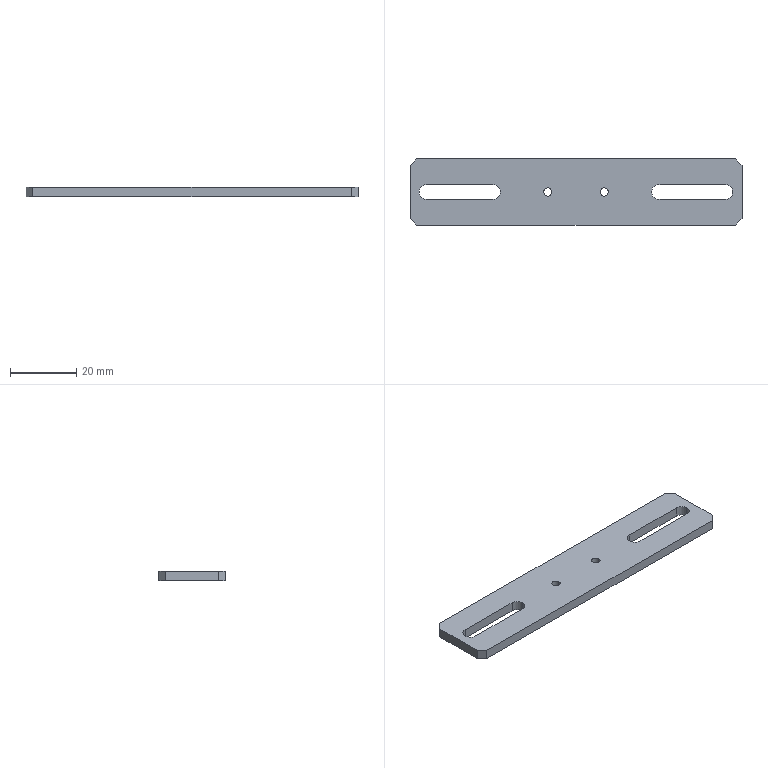Part | SolidWorks | features Chamfer 1, Cut 1, FlatPattern 1, HoleWzd 1, SMBaseFlange 1, SheetMetal 1 | 1 solid | 24 faces | box 100 x 20 x 3 mm | volume 5311 mm3 | plane 14 | cylinder 10 | commonest cylinder face diameters 4.5 x6 2.5 x4
STEP:
#1=CARTESIAN_POINT('',(-22.75,0.,-3.));
#2=VERTEX_POINT('',#1);
#3=CARTESIAN_POINT('',(-25.,2.25,-3.));
#4=VERTEX_POINT('',#3);
#5=CARTESIAN_POINT('',(-25.,0.,-3.));
#6=DIRECTION('',(0.,0.,1.));
#7=DIRECTION('',(1.,0.,0.));
#8=AXIS2_PLACEMENT_3D('',#5,#6,#7);
#9=CIRCLE('',#8,2.25);
#10=EDGE_CURVE('',#2,#4,#9,.T.);
#11=ORIENTED_EDGE('',*,*,#10,.F.);
#12=CARTESIAN_POINT('',(-22.75,0.,0.));
#13=VERTEX_POINT('',#12);
#14=CARTESIAN_POINT('',(-22.75,0.,-3.));
#15=DIRECTION('',(0.,0.,1.));
#16=VECTOR('',#15,1000.);
#17=LINE('',#14,#16);
#18=EDGE_CURVE('',#2,#13,#17,.T.);
#19=ORIENTED_EDGE('',*,*,#18,.T.);
#20=CARTESIAN_POINT('',(-25.,2.25,0.));
#21=VERTEX_POINT('',#20);
#22=CARTESIAN_POINT('',(-25.,0.,0.));
#23=DIRECTION('',(0.,0.,1.));
#24=DIRECTION('',(1.,0.,0.));
#25=AXIS2_PLACEMENT_3D('',#22,#23,#24);
#26=CIRCLE('',#25,2.25);
#27=EDGE_CURVE('',#13,#21,#26,.T.);
#28=ORIENTED_EDGE('',*,*,#27,.T.);
#29=CARTESIAN_POINT('',(-25.,2.25,-3.));
#30=DIRECTION('',(0.,0.,1.));
#31=VECTOR('',#30,1000.);
#32=LINE('',#29,#31);
#33=EDGE_CURVE('',#4,#21,#32,.T.);
#34=ORIENTED_EDGE('',*,*,#33,.F.);
#35=EDGE_LOOP('',(#11,#19,#28,#34));
#36=FACE_OUTER_BOUND('',#35,.T.);
#37=CARTESIAN_POINT('',(-25.,0.,-3.));
#38=DIRECTION('',(0.,0.,1.));
#39=DIRECTION('',(1.,0.,0.));
#40=AXIS2_PLACEMENT_3D('',#37,#38,#39);
#41=CYLINDRICAL_SURFACE('',#40,2.25);
#42=ADVANCED_FACE('',(#36),#41,.F.);
#43=CARTESIAN_POINT('',(47.25,0.,-3.));
#44=VERTEX_POINT('',#43);
#45=CARTESIAN_POINT('',(45.,2.25,-3.));
#46=VERTEX_POINT('',#45);
#47=CARTESIAN_POINT('',(45.,0.,-3.));
#48=DIRECTION('',(0.,0.,1.));
#49=DIRECTION('',(1.,0.,0.));
#50=AXIS2_PLACEMENT_3D('',#47,#48,#49);
#51=CIRCLE('',#50,2.25);
#52=EDGE_CURVE('',#44,#46,#51,.T.);
#53=ORIENTED_EDGE('',*,*,#52,.F.);
#54=CARTESIAN_POINT('',(47.25,0.,0.));
#55=VERTEX_POINT('',#54);
#56=CARTESIAN_POINT('',(47.25,0.,-3.));
#57=DIRECTION('',(0.,0.,1.));
#58=VECTOR('',#57,1000.);
#59=LINE('',#56,#58);
#60=EDGE_CURVE('',#44,#55,#59,.T.);
#61=ORIENTED_EDGE('',*,*,#60,.T.);
#62=CARTESIAN_POINT('',(45.,2.25,0.));
#63=VERTEX_POINT('',#62);
#64=CARTESIAN_POINT('',(45.,0.,0.));
#65=DIRECTION('',(0.,0.,1.));
#66=DIRECTION('',(1.,0.,0.));
#67=AXIS2_PLACEMENT_3D('',#64,#65,#66);
#68=CIRCLE('',#67,2.25);
#69=EDGE_CURVE('',#55,#63,#68,.T.);
#70=ORIENTED_EDGE('',*,*,#69,.T.);
#71=CARTESIAN_POINT('',(45.,2.25,-3.));
#72=DIRECTION('',(0.,0.,1.));
#73=VECTOR('',#72,1000.);
#74=LINE('',#71,#73);
#75=EDGE_CURVE('',#46,#63,#74,.T.);
#76=ORIENTED_EDGE('',*,*,#75,.F.);
#77=EDGE_LOOP('',(#53,#61,#70,#76));
#78=FACE_OUTER_BOUND('',#77,.T.);
#79=CARTESIAN_POINT('',(45.,0.,-3.));
#80=DIRECTION('',(0.,0.,1.));
#81=DIRECTION('',(1.,0.,0.));
#82=AXIS2_PLACEMENT_3D('',#79,#80,#81);
#83=CYLINDRICAL_SURFACE('',#82,2.25);
#84=ADVANCED_FACE('',(#78),#83,.F.);
#85=CARTESIAN_POINT('',(7.25,0.,-3.));
#86=VERTEX_POINT('',#85);
#87=CARTESIAN_POINT('',(9.75,0.,-3.));
#88=VERTEX_POINT('',#87);
#89=CARTESIAN_POINT('',(8.5,0.,-3.));
#90=DIRECTION('',(0.,0.,1.));
#91=DIRECTION('',(1.,0.,0.));
#92=AXIS2_PLACEMENT_3D('',#89,#90,#91);
#93=CIRCLE('',#92,1.25);
#94=EDGE_CURVE('',#86,#88,#93,.T.);
#95=ORIENTED_EDGE('',*,*,#94,.F.);
#96=CARTESIAN_POINT('',(7.25,0.,0.));
#97=VERTEX_POINT('',#96);
#98=CARTESIAN_POINT('',(7.25,0.,0.));
#99=DIRECTION('',(0.,0.,1.));
#100=VECTOR('',#99,1000.);
#101=LINE('',#98,#100);
#102=EDGE_CURVE('',#86,#97,#101,.T.);
#103=ORIENTED_EDGE('',*,*,#102,.T.);
#104=CARTESIAN_POINT('',(9.75,0.,0.));
#105=VERTEX_POINT('',#104);
#106=CARTESIAN_POINT('',(8.5,0.,0.));
#107=DIRECTION('',(0.,0.,1.));
#108=DIRECTION('',(1.,0.,0.));
#109=AXIS2_PLACEMENT_3D('',#106,#107,#108);
#110=CIRCLE('',#109,1.25);
#111=EDGE_CURVE('',#97,#105,#110,.T.);
#112=ORIENTED_EDGE('',*,*,#111,.T.);
#113=CARTESIAN_POINT('',(9.75,0.,0.));
#114=DIRECTION('',(0.,0.,1.));
#115=VECTOR('',#114,1000.);
#116=LINE('',#113,#115);
#117=EDGE_CURVE('',#88,#105,#116,.T.);
#118=ORIENTED_EDGE('',*,*,#117,.F.);
#119=EDGE_LOOP('',(#95,#103,#112,#118));
#120=FACE_OUTER_BOUND('',#119,.T.);
#121=CARTESIAN_POINT('',(8.5,0.,0.));
#122=DIRECTION('',(0.,0.,1.));
#123=DIRECTION('',(1.,0.,0.));
#124=AXIS2_PLACEMENT_3D('',#121,#122,#123);
#125=CYLINDRICAL_SURFACE('',#124,1.25);
#126=ADVANCED_FACE('',(#120),#125,.F.);
#127=CARTESIAN_POINT('',(-9.75,0.,-3.));
#128=VERTEX_POINT('',#127);
#129=CARTESIAN_POINT('',(-7.25,0.,-3.));
#130=VERTEX_POINT('',#129);
#131=CARTESIAN_POINT('',(-8.5,0.,-3.));
#132=DIRECTION('',(0.,0.,1.));
#133=DIRECTION('',(1.,0.,0.));
#134=AXIS2_PLACEMENT_3D('',#131,#132,#133);
#135=CIRCLE('',#134,1.25);
#136=EDGE_CURVE('',#128,#130,#135,.T.);
#137=ORIENTED_EDGE('',*,*,#136,.F.);
#138=CARTESIAN_POINT('',(-9.75,0.,0.));
#139=VERTEX_POINT('',#138);
#140=CARTESIAN_POINT('',(-9.75,0.,0.));
#141=DIRECTION('',(0.,0.,1.));
#142=VECTOR('',#141,1000.);
#143=LINE('',#140,#142);
#144=EDGE_CURVE('',#128,#139,#143,.T.);
#145=ORIENTED_EDGE('',*,*,#144,.T.);
#146=CARTESIAN_POINT('',(-7.25,0.,0.));
#147=VERTEX_POINT('',#146);
#148=CARTESIAN_POINT('',(-8.5,0.,0.));
#149=DIRECTION('',(0.,0.,1.));
#150=DIRECTION('',(1.,0.,0.));
#151=AXIS2_PLACEMENT_3D('',#148,#149,#150);
#152=CIRCLE('',#151,1.25);
#153=EDGE_CURVE('',#139,#147,#152,.T.);
#154=ORIENTED_EDGE('',*,*,#153,.T.);
#155=CARTESIAN_POINT('',(-7.25,0.,0.));
#156=DIRECTION('',(0.,0.,1.));
#157=VECTOR('',#156,1000.);
#158=LINE('',#155,#157);
#159=EDGE_CURVE('',#130,#147,#158,.T.);
#160=ORIENTED_EDGE('',*,*,#159,.F.);
#161=EDGE_LOOP('',(#137,#145,#154,#160));
#162=FACE_OUTER_BOUND('',#161,.T.);
#163=CARTESIAN_POINT('',(-8.5,0.,0.));
#164=DIRECTION('',(0.,0.,1.));
#165=DIRECTION('',(1.,0.,0.));
#166=AXIS2_PLACEMENT_3D('',#163,#164,#165);
#167=CYLINDRICAL_SURFACE('',#166,1.25);
#168=ADVANCED_FACE('',(#162),#167,.F.);
#169=CARTESIAN_POINT('',(50.,-8.,-3.));
#170=VERTEX_POINT('',#169);
#171=CARTESIAN_POINT('',(50.,8.,-3.));
#172=VERTEX_POINT('',#171);
#173=CARTESIAN_POINT('',(50.,10.,-3.));
#174=DIRECTION('',(0.,1.,0.));
#175=VECTOR('',#174,1000.);
#176=LINE('',#173,#175);
#177=EDGE_CURVE('',#170,#172,#176,.T.);
#178=ORIENTED_EDGE('',*,*,#177,.T.);
#179=CARTESIAN_POINT('',(50.,8.,0.));
#180=VERTEX_POINT('',#179);
#181=CARTESIAN_POINT('',(50.,8.,-3.));
#182=DIRECTION('',(0.,0.,1.));
#183=VECTOR('',#182,1000.);
#184=LINE('',#181,#183);
#185=EDGE_CURVE('',#172,#180,#184,.T.);
#186=ORIENTED_EDGE('',*,*,#185,.T.);
#187=CARTESIAN_POINT('',(50.,-8.,0.));
#188=VERTEX_POINT('',#187);
#189=CARTESIAN_POINT('',(50.,10.,0.));
#190=DIRECTION('',(0.,1.,0.));
#191=VECTOR('',#190,1000.);
#192=LINE('',#189,#191);
#193=EDGE_CURVE('',#188,#180,#192,.T.);
#194=ORIENTED_EDGE('',*,*,#193,.F.);
#195=CARTESIAN_POINT('',(50.,-8.,-3.));
#196=DIRECTION('',(0.,0.,-1.));
#197=VECTOR('',#196,1000.);
#198=LINE('',#195,#197);
#199=EDGE_CURVE('',#188,#170,#198,.T.);
#200=ORIENTED_EDGE('',*,*,#199,.T.);
#201=EDGE_LOOP('',(#178,#186,#194,#200));
#202=FACE_OUTER_BOUND('',#201,.T.);
#203=CARTESIAN_POINT('',(50.,10.,-3.));
#204=DIRECTION('',(1.,0.,0.));
#205=DIRECTION('',(0.,0.,-1.));
#206=AXIS2_PLACEMENT_3D('',#203,#204,#205);
#207=PLANE('',#206);
#208=ADVANCED_FACE('',(#202),#207,.T.);
#209=CARTESIAN_POINT('',(-48.,-10.,-3.));
#210=VERTEX_POINT('',#209);
#211=CARTESIAN_POINT('',(48.,-10.,-3.));
#212=VERTEX_POINT('',#211);
#213=CARTESIAN_POINT('',(-50.,-10.,-3.));
#214=DIRECTION('',(1.,0.,0.));
#215=VECTOR('',#214,1000.);
#216=LINE('',#213,#215);
#217=EDGE_CURVE('',#210,#212,#216,.T.);
#218=ORIENTED_EDGE('',*,*,#217,.T.);
#219=CARTESIAN_POINT('',(48.,-10.,0.));
#220=VERTEX_POINT('',#219);
#221=CARTESIAN_POINT('',(48.,-10.,-3.));
#222=DIRECTION('',(0.,0.,1.));
#223=VECTOR('',#222,1000.);
#224=LINE('',#221,#223);
#225=EDGE_CURVE('',#212,#220,#224,.T.);
#226=ORIENTED_EDGE('',*,*,#225,.T.);
#227=CARTESIAN_POINT('',(-48.,-10.,0.));
#228=VERTEX_POINT('',#227);
#229=CARTESIAN_POINT('',(-50.,-10.,0.));
#230=DIRECTION('',(1.,0.,0.));
#231=VECTOR('',#230,1000.);
#232=LINE('',#229,#231);
#233=EDGE_CURVE('',#228,#220,#232,.T.);
#234=ORIENTED_EDGE('',*,*,#233,.F.);
#235=CARTESIAN_POINT('',(-48.,-10.,-3.));
#236=DIRECTION('',(0.,0.,-1.));
#237=VECTOR('',#236,1000.);
#238=LINE('',#235,#237);
#239=EDGE_CURVE('',#228,#210,#238,.T.);
#240=ORIENTED_EDGE('',*,*,#239,.T.);
#241=EDGE_LOOP('',(#218,#226,#234,#240));
#242=FACE_OUTER_BOUND('',#241,.T.);
#243=CARTESIAN_POINT('',(-50.,-10.,-3.));
#244=DIRECTION('',(0.,-1.,0.));
#245=DIRECTION('',(0.,0.,-1.));
#246=AXIS2_PLACEMENT_3D('',#243,#244,#245);
#247=PLANE('',#246);
#248=ADVANCED_FACE('',(#242),#247,.T.);
#249=CARTESIAN_POINT('',(-50.,8.,0.));
#250=VERTEX_POINT('',#249);
#251=CARTESIAN_POINT('',(-50.,-8.,0.));
#252=VERTEX_POINT('',#251);
#253=CARTESIAN_POINT('',(-50.,10.,0.));
#254=DIRECTION('',(0.,-1.,0.));
#255=VECTOR('',#254,1000.);
#256=LINE('',#253,#255);
#257=EDGE_CURVE('',#250,#252,#256,.T.);
#258=ORIENTED_EDGE('',*,*,#257,.F.);
#259=CARTESIAN_POINT('',(-50.,8.,-3.));
#260=VERTEX_POINT('',#259);
#261=CARTESIAN_POINT('',(-50.,8.,-3.));
#262=DIRECTION('',(0.,0.,-1.));
#263=VECTOR('',#262,1000.);
#264=LINE('',#261,#263);
#265=EDGE_CURVE('',#250,#260,#264,.T.);
#266=ORIENTED_EDGE('',*,*,#265,.T.);
#267=CARTESIAN_POINT('',(-50.,-8.,-3.));
#268=VERTEX_POINT('',#267);
#269=CARTESIAN_POINT('',(-50.,10.,-3.));
#270=DIRECTION('',(0.,-1.,0.));
#271=VECTOR('',#270,1000.);
#272=LINE('',#269,#271);
#273=EDGE_CURVE('',#260,#268,#272,.T.);
#274=ORIENTED_EDGE('',*,*,#273,.T.);
#275=CARTESIAN_POINT('',(-50.,-8.,-3.));
#276=DIRECTION('',(0.,0.,1.));
#277=VECTOR('',#276,1000.);
#278=LINE('',#275,#277);
#279=EDGE_CURVE('',#268,#252,#278,.T.);
#280=ORIENTED_EDGE('',*,*,#279,.T.);
#281=EDGE_LOOP('',(#258,#266,#274,#280));
#282=FACE_OUTER_BOUND('',#281,.T.);
#283=CARTESIAN_POINT('',(-50.,10.,-3.));
#284=DIRECTION('',(-1.,0.,0.));
#285=DIRECTION('',(0.,0.,1.));
#286=AXIS2_PLACEMENT_3D('',#283,#284,#285);
#287=PLANE('',#286);
#288=ADVANCED_FACE('',(#282),#287,.T.);
#289=CARTESIAN_POINT('',(48.,10.,0.));
#290=VERTEX_POINT('',#289);
#291=CARTESIAN_POINT('',(-48.,10.,0.));
#292=VERTEX_POINT('',#291);
#293=CARTESIAN_POINT('',(-50.,10.,0.));
#294=DIRECTION('',(-1.,0.,0.));
#295=VECTOR('',#294,1000.);
#296=LINE('',#293,#295);
#297=EDGE_CURVE('',#290,#292,#296,.T.);
#298=ORIENTED_EDGE('',*,*,#297,.F.);
#299=CARTESIAN_POINT('',(48.,10.,-3.));
#300=VERTEX_POINT('',#299);
#301=CARTESIAN_POINT('',(48.,10.,-3.));
#302=DIRECTION('',(0.,0.,-1.));
#303=VECTOR('',#302,1000.);
#304=LINE('',#301,#303);
#305=EDGE_CURVE('',#290,#300,#304,.T.);
#306=ORIENTED_EDGE('',*,*,#305,.T.);
#307=CARTESIAN_POINT('',(-48.,10.,-3.));
#308=VERTEX_POINT('',#307);
#309=CARTESIAN_POINT('',(-50.,10.,-3.));
#310=DIRECTION('',(-1.,0.,0.));
#311=VECTOR('',#310,1000.);
#312=LINE('',#309,#311);
#313=EDGE_CURVE('',#300,#308,#312,.T.);
#314=ORIENTED_EDGE('',*,*,#313,.T.);
#315=CARTESIAN_POINT('',(-48.,10.,-3.));
#316=DIRECTION('',(0.,0.,1.));
#317=VECTOR('',#316,1000.);
#318=LINE('',#315,#317);
#319=EDGE_CURVE('',#308,#292,#318,.T.);
#320=ORIENTED_EDGE('',*,*,#319,.T.);
#321=EDGE_LOOP('',(#298,#306,#314,#320));
#322=FACE_OUTER_BOUND('',#321,.T.);
#323=CARTESIAN_POINT('',(-50.,10.,-3.));
#324=DIRECTION('',(0.,1.,0.));
#325=DIRECTION('',(0.,0.,1.));
#326=AXIS2_PLACEMENT_3D('',#323,#324,#325);
#327=PLANE('',#326);
#328=ADVANCED_FACE('',(#322),#327,.T.);
#329=CARTESIAN_POINT('',(-45.,-2.25,-3.));
#330=VERTEX_POINT('',#329);
#331=CARTESIAN_POINT('',(-25.,-2.25,-3.));
#332=VERTEX_POINT('',#331);
#333=CARTESIAN_POINT('',(-25.,-2.25,-3.));
#334=DIRECTION('',(1.,0.,0.));
#335=VECTOR('',#334,1000.);
#336=LINE('',#333,#335);
#337=EDGE_CURVE('',#330,#332,#336,.T.);
#338=ORIENTED_EDGE('',*,*,#337,.T.);
#339=CARTESIAN_POINT('',(-25.,0.,-3.));
#340=DIRECTION('',(0.,0.,1.));
#341=DIRECTION('',(1.,0.,0.));
#342=AXIS2_PLACEMENT_3D('',#339,#340,#341);
#343=CIRCLE('',#342,2.25);
#344=EDGE_CURVE('',#332,#2,#343,.T.);
#345=ORIENTED_EDGE('',*,*,#344,.T.);
#346=ORIENTED_EDGE('',*,*,#10,.T.);
#347=CARTESIAN_POINT('',(-45.,2.25,-3.));
#348=VERTEX_POINT('',#347);
#349=CARTESIAN_POINT('',(-25.,2.25,-3.));
#350=DIRECTION('',(-1.,0.,0.));
#351=VECTOR('',#350,1000.);
#352=LINE('',#349,#351);
#353=EDGE_CURVE('',#4,#348,#352,.T.);
#354=ORIENTED_EDGE('',*,*,#353,.T.);
#355=CARTESIAN_POINT('',(-45.,0.,-3.));
#356=DIRECTION('',(0.,0.,1.));
#357=DIRECTION('',(1.,0.,0.));
#358=AXIS2_PLACEMENT_3D('',#355,#356,#357);
#359=CIRCLE('',#358,2.25);
#360=EDGE_CURVE('',#348,#330,#359,.T.);
#361=ORIENTED_EDGE('',*,*,#360,.T.);
#362=EDGE_LOOP('',(#338,#345,#346,#354,#361));
#363=FACE_BOUND('',#362,.T.);
#364=CARTESIAN_POINT('',(25.,-2.25,-3.));
#365=VERTEX_POINT('',#364);
#366=CARTESIAN_POINT('',(45.,-2.25,-3.));
#367=VERTEX_POINT('',#366);
#368=CARTESIAN_POINT('',(45.,-2.25,-3.));
#369=DIRECTION('',(1.,0.,0.));
#370=VECTOR('',#369,1000.);
#371=LINE('',#368,#370);
#372=EDGE_CURVE('',#365,#367,#371,.T.);
#373=ORIENTED_EDGE('',*,*,#372,.T.);
#374=CARTESIAN_POINT('',(45.,0.,-3.));
#375=DIRECTION('',(0.,0.,1.));
#376=DIRECTION('',(1.,0.,0.));
#377=AXIS2_PLACEMENT_3D('',#374,#375,#376);
#378=CIRCLE('',#377,2.25);
#379=EDGE_CURVE('',#367,#44,#378,.T.);
#380=ORIENTED_EDGE('',*,*,#379,.T.);
#381=ORIENTED_EDGE('',*,*,#52,.T.);
#382=CARTESIAN_POINT('',(25.,2.25,-3.));
#383=VERTEX_POINT('',#382);
#384=CARTESIAN_POINT('',(45.,2.25,-3.));
#385=DIRECTION('',(-1.,0.,0.));
#386=VECTOR('',#385,1000.);
#387=LINE('',#384,#386);
#388=EDGE_CURVE('',#46,#383,#387,.T.);
#389=ORIENTED_EDGE('',*,*,#388,.T.);
#390=CARTESIAN_POINT('',(25.,0.,-3.));
#391=DIRECTION('',(0.,0.,1.));
#392=DIRECTION('',(1.,0.,0.));
#393=AXIS2_PLACEMENT_3D('',#390,#391,#392);
#394=CIRCLE('',#393,2.25);
#395=EDGE_CURVE('',#383,#365,#394,.T.);
#396=ORIENTED_EDGE('',*,*,#395,.T.);
#397=EDGE_LOOP('',(#373,#380,#381,#389,#396));
#398=FACE_BOUND('',#397,.T.);
#399=CARTESIAN_POINT('',(8.5,0.,-3.));
#400=DIRECTION('',(0.,0.,1.));
#401=DIRECTION('',(1.,0.,0.));
#402=AXIS2_PLACEMENT_3D('',#399,#400,#401);
#403=CIRCLE('',#402,1.25);
#404=EDGE_CURVE('',#88,#86,#403,.T.);
#405=ORIENTED_EDGE('',*,*,#404,.T.);
#406=ORIENTED_EDGE('',*,*,#94,.T.);
#407=EDGE_LOOP('',(#405,#406));
#408=FACE_BOUND('',#407,.T.);
#409=CARTESIAN_POINT('',(-8.5,0.,-3.));
#410=DIRECTION('',(0.,0.,1.));
#411=DIRECTION('',(1.,0.,0.));
#412=AXIS2_PLACEMENT_3D('',#409,#410,#411);
#413=CIRCLE('',#412,1.25);
#414=EDGE_CURVE('',#130,#128,#413,.T.);
#415=ORIENTED_EDGE('',*,*,#414,.T.);
#416=ORIENTED_EDGE('',*,*,#136,.T.);
#417=EDGE_LOOP('',(#415,#416));
#418=FACE_BOUND('',#417,.T.);
#419=ORIENTED_EDGE('',*,*,#313,.F.);
#420=CARTESIAN_POINT('',(50.,8.,-3.));
#421=DIRECTION('',(0.7071,-0.7071,0.));
#422=VECTOR('',#421,1000.);
#423=LINE('',#420,#422);
#424=EDGE_CURVE('',#300,#172,#423,.T.);
#425=ORIENTED_EDGE('',*,*,#424,.T.);
#426=ORIENTED_EDGE('',*,*,#177,.F.);
#427=CARTESIAN_POINT('',(48.,-10.,-3.));
#428=DIRECTION('',(-0.7071,-0.7071,0.));
#429=VECTOR('',#428,1000.);
#430=LINE('',#427,#429);
#431=EDGE_CURVE('',#170,#212,#430,.T.);
#432=ORIENTED_EDGE('',*,*,#431,.T.);
#433=ORIENTED_EDGE('',*,*,#217,.F.);
#434=CARTESIAN_POINT('',(-50.,-8.,-3.));
#435=DIRECTION('',(-0.7071,0.7071,0.));
#436=VECTOR('',#435,1000.);
#437=LINE('',#434,#436);
#438=EDGE_CURVE('',#210,#268,#437,.T.);
#439=ORIENTED_EDGE('',*,*,#438,.T.);
#440=ORIENTED_EDGE('',*,*,#273,.F.);
#441=CARTESIAN_POINT('',(-48.,10.,-3.));
#442=DIRECTION('',(0.7071,0.7071,0.));
#443=VECTOR('',#442,1000.);
#444=LINE('',#441,#443);
#445=EDGE_CURVE('',#260,#308,#444,.T.);
#446=ORIENTED_EDGE('',*,*,#445,.T.);
#447=EDGE_LOOP('',(#419,#425,#426,#432,#433,#439,#440,#446));
#448=FACE_OUTER_BOUND('',#447,.T.);
#449=CARTESIAN_POINT('',(0.,0.,-3.));
#450=DIRECTION('',(0.,0.,1.));
#451=DIRECTION('',(1.,0.,0.));
#452=AXIS2_PLACEMENT_3D('',#449,#450,#451);
#453=PLANE('',#452);
#454=ADVANCED_FACE('',(#363,#398,#408,#418,#448),#453,.F.);
#455=CARTESIAN_POINT('',(-25.,-2.25,0.));
#456=VERTEX_POINT('',#455);
#457=CARTESIAN_POINT('',(-25.,0.,0.));
#458=DIRECTION('',(0.,0.,1.));
#459=DIRECTION('',(1.,0.,0.));
#460=AXIS2_PLACEMENT_3D('',#457,#458,#459);
#461=CIRCLE('',#460,2.25);
#462=EDGE_CURVE('',#456,#13,#461,.T.);
#463=ORIENTED_EDGE('',*,*,#462,.F.);
#464=CARTESIAN_POINT('',(-45.,-2.25,0.));
#465=VERTEX_POINT('',#464);
#466=CARTESIAN_POINT('',(-25.,-2.25,0.));
#467=DIRECTION('',(1.,0.,0.));
#468=VECTOR('',#467,1000.);
#469=LINE('',#466,#468);
#470=EDGE_CURVE('',#465,#456,#469,.T.);
#471=ORIENTED_EDGE('',*,*,#470,.F.);
#472=CARTESIAN_POINT('',(-45.,2.25,0.));
#473=VERTEX_POINT('',#472);
#474=CARTESIAN_POINT('',(-45.,0.,0.));
#475=DIRECTION('',(0.,0.,1.));
#476=DIRECTION('',(1.,0.,0.));
#477=AXIS2_PLACEMENT_3D('',#474,#475,#476);
#478=CIRCLE('',#477,2.25);
#479=EDGE_CURVE('',#473,#465,#478,.T.);
#480=ORIENTED_EDGE('',*,*,#479,.F.);
#481=CARTESIAN_POINT('',(-25.,2.25,0.));
#482=DIRECTION('',(-1.,0.,0.));
#483=VECTOR('',#482,1000.);
#484=LINE('',#481,#483);
#485=EDGE_CURVE('',#21,#473,#484,.T.);
#486=ORIENTED_EDGE('',*,*,#485,.F.);
#487=ORIENTED_EDGE('',*,*,#27,.F.);
#488=EDGE_LOOP('',(#463,#471,#480,#486,#487));
#489=FACE_BOUND('',#488,.T.);
#490=CARTESIAN_POINT('',(45.,-2.25,0.));
#491=VERTEX_POINT('',#490);
#492=CARTESIAN_POINT('',(45.,0.,0.));
#493=DIRECTION('',(0.,0.,1.));
#494=DIRECTION('',(1.,0.,0.));
#495=AXIS2_PLACEMENT_3D('',#492,#493,#494);
#496=CIRCLE('',#495,2.25);
#497=EDGE_CURVE('',#491,#55,#496,.T.);
#498=ORIENTED_EDGE('',*,*,#497,.F.);
#499=CARTESIAN_POINT('',(25.,-2.25,0.));
#500=VERTEX_POINT('',#499);
#501=CARTESIAN_POINT('',(45.,-2.25,0.));
#502=DIRECTION('',(1.,0.,0.));
#503=VECTOR('',#502,1000.);
#504=LINE('',#501,#503);
#505=EDGE_CURVE('',#500,#491,#504,.T.);
#506=ORIENTED_EDGE('',*,*,#505,.F.);
#507=CARTESIAN_POINT('',(25.,2.25,0.));
#508=VERTEX_POINT('',#507);
#509=CARTESIAN_POINT('',(25.,0.,0.));
#510=DIRECTION('',(0.,0.,1.));
#511=DIRECTION('',(1.,0.,0.));
#512=AXIS2_PLACEMENT_3D('',#509,#510,#511);
#513=CIRCLE('',#512,2.25);
#514=EDGE_CURVE('',#508,#500,#513,.T.);
#515=ORIENTED_EDGE('',*,*,#514,.F.);
#516=CARTESIAN_POINT('',(45.,2.25,0.));
#517=DIRECTION('',(-1.,0.,0.));
#518=VECTOR('',#517,1000.);
#519=LINE('',#516,#518);
#520=EDGE_CURVE('',#63,#508,#519,.T.);
#521=ORIENTED_EDGE('',*,*,#520,.F.);
#522=ORIENTED_EDGE('',*,*,#69,.F.);
#523=EDGE_LOOP('',(#498,#506,#515,#521,#522));
#524=FACE_BOUND('',#523,.T.);
#525=CARTESIAN_POINT('',(8.5,0.,0.));
#526=DIRECTION('',(0.,0.,1.));
#527=DIRECTION('',(1.,0.,0.));
#528=AXIS2_PLACEMENT_3D('',#525,#526,#527);
#529=CIRCLE('',#528,1.25);
#530=EDGE_CURVE('',#105,#97,#529,.T.);
#531=ORIENTED_EDGE('',*,*,#530,.F.);
#532=ORIENTED_EDGE('',*,*,#111,.F.);
#533=EDGE_LOOP('',(#531,#532));
#534=FACE_BOUND('',#533,.T.);
#535=CARTESIAN_POINT('',(-8.5,0.,0.));
#536=DIRECTION('',(0.,0.,1.));
#537=DIRECTION('',(1.,0.,0.));
#538=AXIS2_PLACEMENT_3D('',#535,#536,#537);
#539=CIRCLE('',#538,1.25);
#540=EDGE_CURVE('',#147,#139,#539,.T.);
#541=ORIENTED_EDGE('',*,*,#540,.F.);
#542=ORIENTED_EDGE('',*,*,#153,.F.);
#543=EDGE_LOOP('',(#541,#542));
#544=FACE_BOUND('',#543,.T.);
#545=ORIENTED_EDGE('',*,*,#193,.T.);
#546=CARTESIAN_POINT('',(29.,29.,0.));
#547=DIRECTION('',(-0.7071,0.7071,0.));
#548=VECTOR('',#547,1000.);
#549=LINE('',#546,#548);
#550=EDGE_CURVE('',#180,#290,#549,.T.);
#551=ORIENTED_EDGE('',*,*,#550,.T.);
#552=ORIENTED_EDGE('',*,*,#297,.T.);
#553=CARTESIAN_POINT('',(-29.,29.,0.));
#554=DIRECTION('',(-0.7071,-0.7071,0.));
#555=VECTOR('',#554,1000.);
#556=LINE('',#553,#555);
#557=EDGE_CURVE('',#292,#250,#556,.T.);
#558=ORIENTED_EDGE('',*,*,#557,.T.);
#559=ORIENTED_EDGE('',*,*,#257,.T.);
#560=CARTESIAN_POINT('',(-29.,-29.,0.));
#561=DIRECTION('',(0.7071,-0.7071,0.));
#562=VECTOR('',#561,1000.);
#563=LINE('',#560,#562);
#564=EDGE_CURVE('',#252,#228,#563,.T.);
#565=ORIENTED_EDGE('',*,*,#564,.T.);
#566=ORIENTED_EDGE('',*,*,#233,.T.);
#567=CARTESIAN_POINT('',(29.,-29.,0.));
#568=DIRECTION('',(0.7071,0.7071,0.));
#569=VECTOR('',#568,1000.);
#570=LINE('',#567,#569);
#571=EDGE_CURVE('',#220,#188,#570,.T.);
#572=ORIENTED_EDGE('',*,*,#571,.T.);
#573=EDGE_LOOP('',(#545,#551,#552,#558,#559,#565,#566,#572));
#574=FACE_OUTER_BOUND('',#573,.T.);
#575=CARTESIAN_POINT('',(0.,0.,0.));
#576=DIRECTION('',(0.,0.,1.));
#577=DIRECTION('',(1.,0.,0.));
#578=AXIS2_PLACEMENT_3D('',#575,#576,#577);
#579=PLANE('',#578);
#580=ADVANCED_FACE('',(#489,#524,#534,#544,#574),#579,.T.);
#581=ORIENTED_EDGE('',*,*,#144,.F.);
#582=ORIENTED_EDGE('',*,*,#414,.F.);
#583=ORIENTED_EDGE('',*,*,#159,.T.);
#584=ORIENTED_EDGE('',*,*,#540,.T.);
#585=EDGE_LOOP('',(#581,#582,#583,#584));
#586=FACE_OUTER_BOUND('',#585,.T.);
#587=CARTESIAN_POINT('',(-8.5,0.,0.));
#588=DIRECTION('',(0.,0.,1.));
#589=DIRECTION('',(1.,0.,0.));
#590=AXIS2_PLACEMENT_3D('',#587,#588,#589);
#591=CYLINDRICAL_SURFACE('',#590,1.25);
#592=ADVANCED_FACE('',(#586),#591,.F.);
#593=ORIENTED_EDGE('',*,*,#102,.F.);
#594=ORIENTED_EDGE('',*,*,#404,.F.);
#595=ORIENTED_EDGE('',*,*,#117,.T.);
#596=ORIENTED_EDGE('',*,*,#530,.T.);
#597=EDGE_LOOP('',(#593,#594,#595,#596));
#598=FACE_OUTER_BOUND('',#597,.T.);
#599=CARTESIAN_POINT('',(8.5,0.,0.));
#600=DIRECTION('',(0.,0.,1.));
#601=DIRECTION('',(1.,0.,0.));
#602=AXIS2_PLACEMENT_3D('',#599,#600,#601);
#603=CYLINDRICAL_SURFACE('',#602,1.25);
#604=ADVANCED_FACE('',(#598),#603,.F.);
#605=ORIENTED_EDGE('',*,*,#60,.F.);
#606=ORIENTED_EDGE('',*,*,#379,.F.);
#607=CARTESIAN_POINT('',(45.,-2.25,-3.));
#608=DIRECTION('',(0.,0.,1.));
#609=VECTOR('',#608,1000.);
#610=LINE('',#607,#609);
#611=EDGE_CURVE('',#367,#491,#610,.T.);
#612=ORIENTED_EDGE('',*,*,#611,.T.);
#613=ORIENTED_EDGE('',*,*,#497,.T.);
#614=EDGE_LOOP('',(#605,#606,#612,#613));
#615=FACE_OUTER_BOUND('',#614,.T.);
#616=CARTESIAN_POINT('',(45.,0.,-3.));
#617=DIRECTION('',(0.,0.,1.));
#618=DIRECTION('',(1.,0.,0.));
#619=AXIS2_PLACEMENT_3D('',#616,#617,#618);
#620=CYLINDRICAL_SURFACE('',#619,2.25);
#621=ADVANCED_FACE('',(#615),#620,.F.);
#622=ORIENTED_EDGE('',*,*,#505,.T.);
#623=ORIENTED_EDGE('',*,*,#611,.F.);
#624=ORIENTED_EDGE('',*,*,#372,.F.);
#625=CARTESIAN_POINT('',(25.,-2.25,-3.));
#626=DIRECTION('',(0.,0.,1.));
#627=VECTOR('',#626,1000.);
#628=LINE('',#625,#627);
#629=EDGE_CURVE('',#365,#500,#628,.T.);
#630=ORIENTED_EDGE('',*,*,#629,.T.);
#631=EDGE_LOOP('',(#622,#623,#624,#630));
#632=FACE_OUTER_BOUND('',#631,.T.);
#633=CARTESIAN_POINT('',(45.,-2.25,-3.));
#634=DIRECTION('',(0.,-1.,0.));
#635=DIRECTION('',(1.,0.,0.));
#636=AXIS2_PLACEMENT_3D('',#633,#634,#635);
#637=PLANE('',#636);
#638=ADVANCED_FACE('',(#632),#637,.F.);
#639=ORIENTED_EDGE('',*,*,#514,.T.);
#640=ORIENTED_EDGE('',*,*,#629,.F.);
#641=ORIENTED_EDGE('',*,*,#395,.F.);
#642=CARTESIAN_POINT('',(25.,2.25,-3.));
#643=DIRECTION('',(0.,0.,1.));
#644=VECTOR('',#643,1000.);
#645=LINE('',#642,#644);
#646=EDGE_CURVE('',#383,#508,#645,.T.);
#647=ORIENTED_EDGE('',*,*,#646,.T.);
#648=EDGE_LOOP('',(#639,#640,#641,#647));
#649=FACE_OUTER_BOUND('',#648,.T.);
#650=CARTESIAN_POINT('',(25.,0.,-3.));
#651=DIRECTION('',(0.,0.,1.));
#652=DIRECTION('',(1.,0.,0.));
#653=AXIS2_PLACEMENT_3D('',#650,#651,#652);
#654=CYLINDRICAL_SURFACE('',#653,2.25);
#655=ADVANCED_FACE('',(#649),#654,.F.);
#656=ORIENTED_EDGE('',*,*,#520,.T.);
#657=ORIENTED_EDGE('',*,*,#646,.F.);
#658=ORIENTED_EDGE('',*,*,#388,.F.);
#659=ORIENTED_EDGE('',*,*,#75,.T.);
#660=EDGE_LOOP('',(#656,#657,#658,#659));
#661=FACE_OUTER_BOUND('',#660,.T.);
#662=CARTESIAN_POINT('',(45.,2.25,-3.));
#663=DIRECTION('',(0.,1.,0.));
#664=DIRECTION('',(-1.,0.,0.));
#665=AXIS2_PLACEMENT_3D('',#662,#663,#664);
#666=PLANE('',#665);
#667=ADVANCED_FACE('',(#661),#666,.F.);
#668=ORIENTED_EDGE('',*,*,#18,.F.);
#669=ORIENTED_EDGE('',*,*,#344,.F.);
#670=CARTESIAN_POINT('',(-25.,-2.25,-3.));
#671=DIRECTION('',(0.,0.,1.));
#672=VECTOR('',#671,1000.);
#673=LINE('',#670,#672);
#674=EDGE_CURVE('',#332,#456,#673,.T.);
#675=ORIENTED_EDGE('',*,*,#674,.T.);
#676=ORIENTED_EDGE('',*,*,#462,.T.);
#677=EDGE_LOOP('',(#668,#669,#675,#676));
#678=FACE_OUTER_BOUND('',#677,.T.);
#679=CARTESIAN_POINT('',(-25.,0.,-3.));
#680=DIRECTION('',(0.,0.,1.));
#681=DIRECTION('',(1.,0.,0.));
#682=AXIS2_PLACEMENT_3D('',#679,#680,#681);
#683=CYLINDRICAL_SURFACE('',#682,2.25);
#684=ADVANCED_FACE('',(#678),#683,.F.);
#685=ORIENTED_EDGE('',*,*,#470,.T.);
#686=ORIENTED_EDGE('',*,*,#674,.F.);
#687=ORIENTED_EDGE('',*,*,#337,.F.);
#688=CARTESIAN_POINT('',(-45.,-2.25,-3.));
#689=DIRECTION('',(0.,0.,1.));
#690=VECTOR('',#689,1000.);
#691=LINE('',#688,#690);
#692=EDGE_CURVE('',#330,#465,#691,.T.);
#693=ORIENTED_EDGE('',*,*,#692,.T.);
#694=EDGE_LOOP('',(#685,#686,#687,#693));
#695=FACE_OUTER_BOUND('',#694,.T.);
#696=CARTESIAN_POINT('',(-25.,-2.25,-3.));
#697=DIRECTION('',(0.,-1.,0.));
#698=DIRECTION('',(1.,0.,0.));
#699=AXIS2_PLACEMENT_3D('',#696,#697,#698);
#700=PLANE('',#699);
#701=ADVANCED_FACE('',(#695),#700,.F.);
#702=ORIENTED_EDGE('',*,*,#479,.T.);
#703=ORIENTED_EDGE('',*,*,#692,.F.);
#704=ORIENTED_EDGE('',*,*,#360,.F.);
#705=CARTESIAN_POINT('',(-45.,2.25,-3.));
#706=DIRECTION('',(0.,0.,1.));
#707=VECTOR('',#706,1000.);
#708=LINE('',#705,#707);
#709=EDGE_CURVE('',#348,#473,#708,.T.);
#710=ORIENTED_EDGE('',*,*,#709,.T.);
#711=EDGE_LOOP('',(#702,#703,#704,#710));
#712=FACE_OUTER_BOUND('',#711,.T.);
#713=CARTESIAN_POINT('',(-45.,0.,-3.));
#714=DIRECTION('',(0.,0.,1.));
#715=DIRECTION('',(1.,0.,0.));
#716=AXIS2_PLACEMENT_3D('',#713,#714,#715);
#717=CYLINDRICAL_SURFACE('',#716,2.25);
#718=ADVANCED_FACE('',(#712),#717,.F.);
#719=ORIENTED_EDGE('',*,*,#485,.T.);
#720=ORIENTED_EDGE('',*,*,#709,.F.);
#721=ORIENTED_EDGE('',*,*,#353,.F.);
#722=ORIENTED_EDGE('',*,*,#33,.T.);
#723=EDGE_LOOP('',(#719,#720,#721,#722));
#724=FACE_OUTER_BOUND('',#723,.T.);
#725=CARTESIAN_POINT('',(-25.,2.25,-3.));
#726=DIRECTION('',(0.,1.,0.));
#727=DIRECTION('',(-1.,0.,0.));
#728=AXIS2_PLACEMENT_3D('',#725,#726,#727);
#729=PLANE('',#728);
#730=ADVANCED_FACE('',(#724),#729,.F.);
#731=ORIENTED_EDGE('',*,*,#424,.F.);
#732=ORIENTED_EDGE('',*,*,#305,.F.);
#733=ORIENTED_EDGE('',*,*,#550,.F.);
#734=ORIENTED_EDGE('',*,*,#185,.F.);
#735=EDGE_LOOP('',(#731,#732,#733,#734));
#736=FACE_OUTER_BOUND('',#735,.T.);
#737=CARTESIAN_POINT('',(50.,8.,-3.));
#738=DIRECTION('',(-0.7071,-0.7071,0.));
#739=DIRECTION('',(0.,0.,1.));
#740=AXIS2_PLACEMENT_3D('',#737,#738,#739);
#741=PLANE('',#740);
#742=ADVANCED_FACE('',(#736),#741,.F.);
#743=ORIENTED_EDGE('',*,*,#431,.F.);
#744=ORIENTED_EDGE('',*,*,#199,.F.);
#745=ORIENTED_EDGE('',*,*,#571,.F.);
#746=ORIENTED_EDGE('',*,*,#225,.F.);
#747=EDGE_LOOP('',(#743,#744,#745,#746));
#748=FACE_OUTER_BOUND('',#747,.T.);
#749=CARTESIAN_POINT('',(48.,-10.,-3.));
#750=DIRECTION('',(-0.7071,0.7071,0.));
#751=DIRECTION('',(0.,0.,1.));
#752=AXIS2_PLACEMENT_3D('',#749,#750,#751);
#753=PLANE('',#752);
#754=ADVANCED_FACE('',(#748),#753,.F.);
#755=ORIENTED_EDGE('',*,*,#445,.F.);
#756=ORIENTED_EDGE('',*,*,#265,.F.);
#757=ORIENTED_EDGE('',*,*,#557,.F.);
#758=ORIENTED_EDGE('',*,*,#319,.F.);
#759=EDGE_LOOP('',(#755,#756,#757,#758));
#760=FACE_OUTER_BOUND('',#759,.T.);
#761=CARTESIAN_POINT('',(-48.,10.,-3.));
#762=DIRECTION('',(0.7071,-0.7071,0.));
#763=DIRECTION('',(0.,0.,1.));
#764=AXIS2_PLACEMENT_3D('',#761,#762,#763);
#765=PLANE('',#764);
#766=ADVANCED_FACE('',(#760),#765,.F.);
#767=ORIENTED_EDGE('',*,*,#438,.F.);
#768=ORIENTED_EDGE('',*,*,#239,.F.);
#769=ORIENTED_EDGE('',*,*,#564,.F.);
#770=ORIENTED_EDGE('',*,*,#279,.F.);
#771=EDGE_LOOP('',(#767,#768,#769,#770));
#772=FACE_OUTER_BOUND('',#771,.T.);
#773=CARTESIAN_POINT('',(-50.,-8.,-3.));
#774=DIRECTION('',(0.7071,0.7071,0.));
#775=DIRECTION('',(0.,0.,1.));
#776=AXIS2_PLACEMENT_3D('',#773,#774,#775);
#777=PLANE('',#776);
#778=ADVANCED_FACE('',(#772),#777,.F.);
#779=CLOSED_SHELL('',(#42,#84,#126,#168,#208,#248,#288,#328,#454,#580,#592,#604,#621,#638,#655,#667,#684,#701,#718,#730,#742,#754,#766,#778));
#780=MANIFOLD_SOLID_BREP('',#779);
#781=CARTESIAN_POINT('',(0.,0.,0.));
#782=DIRECTION('',(0.,0.,1.));
#783=DIRECTION('',(1.,0.,0.));
#784=AXIS2_PLACEMENT_3D('',#781,#782,#783);
#785=(LENGTH_UNIT()NAMED_UNIT(*)SI_UNIT(.MILLI.,.METRE.));
#786=UNCERTAINTY_MEASURE_WITH_UNIT(LENGTH_MEASURE(0.00001),#785,'','');
#787=(NAMED_UNIT(*)PLANE_ANGLE_UNIT()SI_UNIT($,.RADIAN.));
#788=(NAMED_UNIT(*)SI_UNIT($,.STERADIAN.)SOLID_ANGLE_UNIT());
#789=(GEOMETRIC_REPRESENTATION_CONTEXT(3)GLOBAL_UNCERTAINTY_ASSIGNED_CONTEXT((#786))GLOBAL_UNIT_ASSIGNED_CONTEXT((#785,#787,#788))REPRESENTATION_CONTEXT('',''));
#790=ADVANCED_BREP_SHAPE_REPRESENTATION('',(#780,#784),#789);